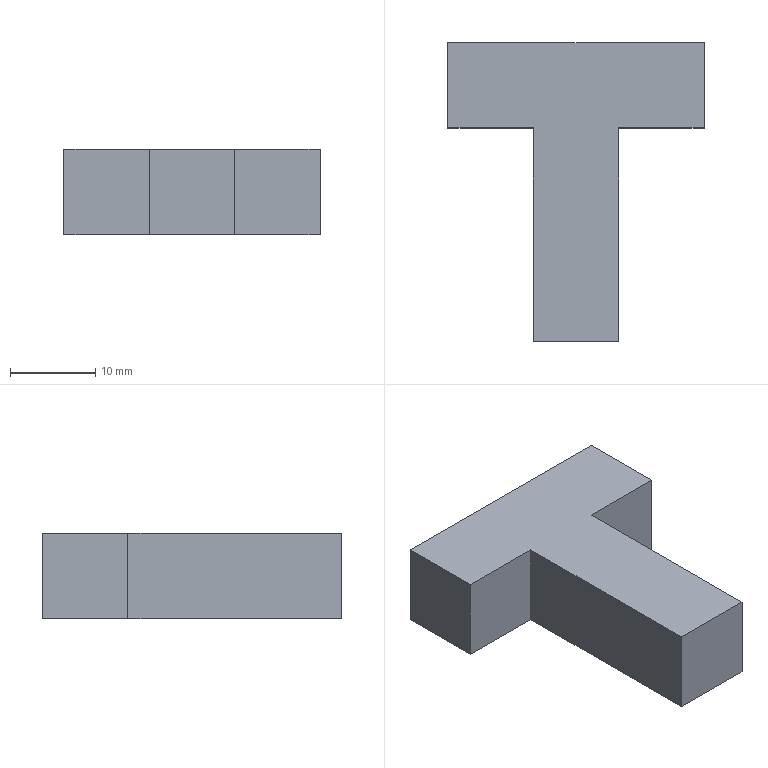Part | SolidWorks | features Extrusion 1, ICE 1 | 1 solid | 10 faces | box 30 x 35 x 10 mm | volume 5500 mm3 | plane 10
STEP:
#1=CARTESIAN_POINT('',(-15.,17.5,0.));
#2=VERTEX_POINT('',#1);
#3=CARTESIAN_POINT('',(-15.,7.5,0.));
#4=VERTEX_POINT('',#3);
#5=CARTESIAN_POINT('',(-15.,17.5,0.));
#6=DIRECTION('',(0.,-1.,0.));
#7=VECTOR('',#6,1000.);
#8=LINE('',#5,#7);
#9=EDGE_CURVE('',#2,#4,#8,.T.);
#10=ORIENTED_EDGE('',*,*,#9,.T.);
#11=CARTESIAN_POINT('',(-15.,7.5,10.));
#12=VERTEX_POINT('',#11);
#13=CARTESIAN_POINT('',(-15.,7.5,0.));
#14=DIRECTION('',(0.,0.,1.));
#15=VECTOR('',#14,1000.);
#16=LINE('',#13,#15);
#17=EDGE_CURVE('',#4,#12,#16,.T.);
#18=ORIENTED_EDGE('',*,*,#17,.T.);
#19=CARTESIAN_POINT('',(-15.,17.5,10.));
#20=VERTEX_POINT('',#19);
#21=CARTESIAN_POINT('',(-15.,17.5,10.));
#22=DIRECTION('',(0.,-1.,0.));
#23=VECTOR('',#22,1000.);
#24=LINE('',#21,#23);
#25=EDGE_CURVE('',#20,#12,#24,.T.);
#26=ORIENTED_EDGE('',*,*,#25,.F.);
#27=CARTESIAN_POINT('',(-15.,17.5,10.));
#28=DIRECTION('',(0.,0.,-1.));
#29=VECTOR('',#28,1000.);
#30=LINE('',#27,#29);
#31=EDGE_CURVE('',#20,#2,#30,.T.);
#32=ORIENTED_EDGE('',*,*,#31,.T.);
#33=EDGE_LOOP('',(#10,#18,#26,#32));
#34=FACE_OUTER_BOUND('',#33,.T.);
#35=CARTESIAN_POINT('',(-15.,17.5,10.));
#36=DIRECTION('',(1.,0.,0.));
#37=DIRECTION('',(0.,1.,0.));
#38=AXIS2_PLACEMENT_3D('',#35,#36,#37);
#39=PLANE('',#38);
#40=ADVANCED_FACE('',(#34),#39,.F.);
#41=CARTESIAN_POINT('',(-5.,-17.5,0.));
#42=VERTEX_POINT('',#41);
#43=CARTESIAN_POINT('',(5.,-17.5,0.));
#44=VERTEX_POINT('',#43);
#45=CARTESIAN_POINT('',(-15.,-17.5,0.));
#46=DIRECTION('',(1.,0.,0.));
#47=VECTOR('',#46,1000.);
#48=LINE('',#45,#47);
#49=EDGE_CURVE('',#42,#44,#48,.T.);
#50=ORIENTED_EDGE('',*,*,#49,.T.);
#51=CARTESIAN_POINT('',(5.,-17.5,10.));
#52=VERTEX_POINT('',#51);
#53=CARTESIAN_POINT('',(5.,-17.5,0.));
#54=DIRECTION('',(0.,0.,1.));
#55=VECTOR('',#54,1000.);
#56=LINE('',#53,#55);
#57=EDGE_CURVE('',#44,#52,#56,.T.);
#58=ORIENTED_EDGE('',*,*,#57,.T.);
#59=CARTESIAN_POINT('',(-5.,-17.5,10.));
#60=VERTEX_POINT('',#59);
#61=CARTESIAN_POINT('',(-15.,-17.5,10.));
#62=DIRECTION('',(1.,0.,0.));
#63=VECTOR('',#62,1000.);
#64=LINE('',#61,#63);
#65=EDGE_CURVE('',#60,#52,#64,.T.);
#66=ORIENTED_EDGE('',*,*,#65,.F.);
#67=CARTESIAN_POINT('',(-5.,-17.5,0.));
#68=DIRECTION('',(0.,0.,1.));
#69=VECTOR('',#68,1000.);
#70=LINE('',#67,#69);
#71=EDGE_CURVE('',#42,#60,#70,.T.);
#72=ORIENTED_EDGE('',*,*,#71,.F.);
#73=EDGE_LOOP('',(#50,#58,#66,#72));
#74=FACE_OUTER_BOUND('',#73,.T.);
#75=CARTESIAN_POINT('',(-15.,-17.5,10.));
#76=DIRECTION('',(0.,1.,0.));
#77=DIRECTION('',(0.,0.,1.));
#78=AXIS2_PLACEMENT_3D('',#75,#76,#77);
#79=PLANE('',#78);
#80=ADVANCED_FACE('',(#74),#79,.F.);
#81=CARTESIAN_POINT('',(15.,7.5,10.));
#82=VERTEX_POINT('',#81);
#83=CARTESIAN_POINT('',(15.,17.5,10.));
#84=VERTEX_POINT('',#83);
#85=CARTESIAN_POINT('',(15.,17.5,10.));
#86=DIRECTION('',(0.,1.,0.));
#87=VECTOR('',#86,1000.);
#88=LINE('',#85,#87);
#89=EDGE_CURVE('',#82,#84,#88,.T.);
#90=ORIENTED_EDGE('',*,*,#89,.F.);
#91=CARTESIAN_POINT('',(15.,7.5,0.));
#92=VERTEX_POINT('',#91);
#93=CARTESIAN_POINT('',(15.,7.5,0.));
#94=DIRECTION('',(0.,0.,1.));
#95=VECTOR('',#94,1000.);
#96=LINE('',#93,#95);
#97=EDGE_CURVE('',#92,#82,#96,.T.);
#98=ORIENTED_EDGE('',*,*,#97,.F.);
#99=CARTESIAN_POINT('',(15.,17.5,0.));
#100=VERTEX_POINT('',#99);
#101=CARTESIAN_POINT('',(15.,17.5,0.));
#102=DIRECTION('',(0.,1.,0.));
#103=VECTOR('',#102,1000.);
#104=LINE('',#101,#103);
#105=EDGE_CURVE('',#92,#100,#104,.T.);
#106=ORIENTED_EDGE('',*,*,#105,.T.);
#107=CARTESIAN_POINT('',(15.,17.5,10.));
#108=DIRECTION('',(0.,0.,-1.));
#109=VECTOR('',#108,1000.);
#110=LINE('',#107,#109);
#111=EDGE_CURVE('',#84,#100,#110,.T.);
#112=ORIENTED_EDGE('',*,*,#111,.F.);
#113=EDGE_LOOP('',(#90,#98,#106,#112));
#114=FACE_OUTER_BOUND('',#113,.T.);
#115=CARTESIAN_POINT('',(15.,17.5,10.));
#116=DIRECTION('',(-1.,0.,0.));
#117=DIRECTION('',(0.,-1.,0.));
#118=AXIS2_PLACEMENT_3D('',#115,#116,#117);
#119=PLANE('',#118);
#120=ADVANCED_FACE('',(#114),#119,.F.);
#121=CARTESIAN_POINT('',(-15.,17.5,0.));
#122=DIRECTION('',(-1.,0.,0.));
#123=VECTOR('',#122,1000.);
#124=LINE('',#121,#123);
#125=EDGE_CURVE('',#100,#2,#124,.T.);
#126=ORIENTED_EDGE('',*,*,#125,.T.);
#127=ORIENTED_EDGE('',*,*,#31,.F.);
#128=CARTESIAN_POINT('',(-15.,17.5,10.));
#129=DIRECTION('',(-1.,0.,0.));
#130=VECTOR('',#129,1000.);
#131=LINE('',#128,#130);
#132=EDGE_CURVE('',#84,#20,#131,.T.);
#133=ORIENTED_EDGE('',*,*,#132,.F.);
#134=ORIENTED_EDGE('',*,*,#111,.T.);
#135=EDGE_LOOP('',(#126,#127,#133,#134));
#136=FACE_OUTER_BOUND('',#135,.T.);
#137=CARTESIAN_POINT('',(-15.,17.5,10.));
#138=DIRECTION('',(0.,-1.,0.));
#139=DIRECTION('',(0.,0.,-1.));
#140=AXIS2_PLACEMENT_3D('',#137,#138,#139);
#141=PLANE('',#140);
#142=ADVANCED_FACE('',(#136),#141,.F.);
#143=CARTESIAN_POINT('',(5.,7.5,10.));
#144=VERTEX_POINT('',#143);
#145=CARTESIAN_POINT('',(5.,-17.5,10.));
#146=DIRECTION('',(0.,-1.,0.));
#147=VECTOR('',#146,1000.);
#148=LINE('',#145,#147);
#149=EDGE_CURVE('',#144,#52,#148,.T.);
#150=ORIENTED_EDGE('',*,*,#149,.F.);
#151=CARTESIAN_POINT('',(15.,7.5,10.));
#152=DIRECTION('',(-1.,0.,0.));
#153=VECTOR('',#152,1000.);
#154=LINE('',#151,#153);
#155=EDGE_CURVE('',#82,#144,#154,.T.);
#156=ORIENTED_EDGE('',*,*,#155,.F.);
#157=ORIENTED_EDGE('',*,*,#89,.T.);
#158=ORIENTED_EDGE('',*,*,#132,.T.);
#159=ORIENTED_EDGE('',*,*,#25,.T.);
#160=CARTESIAN_POINT('',(-5.,7.5,10.));
#161=VERTEX_POINT('',#160);
#162=CARTESIAN_POINT('',(-15.,7.5,10.));
#163=DIRECTION('',(-1.,0.,0.));
#164=VECTOR('',#163,1000.);
#165=LINE('',#162,#164);
#166=EDGE_CURVE('',#161,#12,#165,.T.);
#167=ORIENTED_EDGE('',*,*,#166,.F.);
#168=CARTESIAN_POINT('',(-5.,-17.5,10.));
#169=DIRECTION('',(0.,1.,0.));
#170=VECTOR('',#169,1000.);
#171=LINE('',#168,#170);
#172=EDGE_CURVE('',#60,#161,#171,.T.);
#173=ORIENTED_EDGE('',*,*,#172,.F.);
#174=ORIENTED_EDGE('',*,*,#65,.T.);
#175=EDGE_LOOP('',(#150,#156,#157,#158,#159,#167,#173,#174));
#176=FACE_OUTER_BOUND('',#175,.T.);
#177=CARTESIAN_POINT('',(0.,0.,10.));
#178=DIRECTION('',(0.,0.,1.));
#179=DIRECTION('',(1.,0.,0.));
#180=AXIS2_PLACEMENT_3D('',#177,#178,#179);
#181=PLANE('',#180);
#182=ADVANCED_FACE('',(#176),#181,.T.);
#183=CARTESIAN_POINT('',(5.,7.5,0.));
#184=VERTEX_POINT('',#183);
#185=CARTESIAN_POINT('',(15.,7.5,0.));
#186=DIRECTION('',(-1.,0.,0.));
#187=VECTOR('',#186,1000.);
#188=LINE('',#185,#187);
#189=EDGE_CURVE('',#92,#184,#188,.T.);
#190=ORIENTED_EDGE('',*,*,#189,.T.);
#191=CARTESIAN_POINT('',(5.,-17.5,0.));
#192=DIRECTION('',(0.,-1.,0.));
#193=VECTOR('',#192,1000.);
#194=LINE('',#191,#193);
#195=EDGE_CURVE('',#184,#44,#194,.T.);
#196=ORIENTED_EDGE('',*,*,#195,.T.);
#197=ORIENTED_EDGE('',*,*,#49,.F.);
#198=CARTESIAN_POINT('',(-5.,7.5,0.));
#199=VERTEX_POINT('',#198);
#200=CARTESIAN_POINT('',(-5.,-17.5,0.));
#201=DIRECTION('',(0.,1.,0.));
#202=VECTOR('',#201,1000.);
#203=LINE('',#200,#202);
#204=EDGE_CURVE('',#42,#199,#203,.T.);
#205=ORIENTED_EDGE('',*,*,#204,.T.);
#206=CARTESIAN_POINT('',(-15.,7.5,0.));
#207=DIRECTION('',(-1.,0.,0.));
#208=VECTOR('',#207,1000.);
#209=LINE('',#206,#208);
#210=EDGE_CURVE('',#199,#4,#209,.T.);
#211=ORIENTED_EDGE('',*,*,#210,.T.);
#212=ORIENTED_EDGE('',*,*,#9,.F.);
#213=ORIENTED_EDGE('',*,*,#125,.F.);
#214=ORIENTED_EDGE('',*,*,#105,.F.);
#215=EDGE_LOOP('',(#190,#196,#197,#205,#211,#212,#213,#214));
#216=FACE_OUTER_BOUND('',#215,.T.);
#217=CARTESIAN_POINT('',(0.,0.,0.));
#218=DIRECTION('',(0.,0.,1.));
#219=DIRECTION('',(1.,0.,0.));
#220=AXIS2_PLACEMENT_3D('',#217,#218,#219);
#221=PLANE('',#220);
#222=ADVANCED_FACE('',(#216),#221,.F.);
#223=ORIENTED_EDGE('',*,*,#166,.T.);
#224=ORIENTED_EDGE('',*,*,#17,.F.);
#225=ORIENTED_EDGE('',*,*,#210,.F.);
#226=CARTESIAN_POINT('',(-5.,7.5,0.));
#227=DIRECTION('',(0.,0.,1.));
#228=VECTOR('',#227,1000.);
#229=LINE('',#226,#228);
#230=EDGE_CURVE('',#199,#161,#229,.T.);
#231=ORIENTED_EDGE('',*,*,#230,.T.);
#232=EDGE_LOOP('',(#223,#224,#225,#231));
#233=FACE_OUTER_BOUND('',#232,.T.);
#234=CARTESIAN_POINT('',(-15.,7.5,0.));
#235=DIRECTION('',(0.,1.,0.));
#236=DIRECTION('',(0.,0.,1.));
#237=AXIS2_PLACEMENT_3D('',#234,#235,#236);
#238=PLANE('',#237);
#239=ADVANCED_FACE('',(#233),#238,.F.);
#240=ORIENTED_EDGE('',*,*,#172,.T.);
#241=ORIENTED_EDGE('',*,*,#230,.F.);
#242=ORIENTED_EDGE('',*,*,#204,.F.);
#243=ORIENTED_EDGE('',*,*,#71,.T.);
#244=EDGE_LOOP('',(#240,#241,#242,#243));
#245=FACE_OUTER_BOUND('',#244,.T.);
#246=CARTESIAN_POINT('',(-5.,-17.5,0.));
#247=DIRECTION('',(1.,0.,0.));
#248=DIRECTION('',(0.,0.,-1.));
#249=AXIS2_PLACEMENT_3D('',#246,#247,#248);
#250=PLANE('',#249);
#251=ADVANCED_FACE('',(#245),#250,.F.);
#252=ORIENTED_EDGE('',*,*,#149,.T.);
#253=ORIENTED_EDGE('',*,*,#57,.F.);
#254=ORIENTED_EDGE('',*,*,#195,.F.);
#255=CARTESIAN_POINT('',(5.,7.5,0.));
#256=DIRECTION('',(0.,0.,1.));
#257=VECTOR('',#256,1000.);
#258=LINE('',#255,#257);
#259=EDGE_CURVE('',#184,#144,#258,.T.);
#260=ORIENTED_EDGE('',*,*,#259,.T.);
#261=EDGE_LOOP('',(#252,#253,#254,#260));
#262=FACE_OUTER_BOUND('',#261,.T.);
#263=CARTESIAN_POINT('',(5.,-17.5,0.));
#264=DIRECTION('',(-1.,0.,0.));
#265=DIRECTION('',(0.,0.,1.));
#266=AXIS2_PLACEMENT_3D('',#263,#264,#265);
#267=PLANE('',#266);
#268=ADVANCED_FACE('',(#262),#267,.F.);
#269=ORIENTED_EDGE('',*,*,#155,.T.);
#270=ORIENTED_EDGE('',*,*,#259,.F.);
#271=ORIENTED_EDGE('',*,*,#189,.F.);
#272=ORIENTED_EDGE('',*,*,#97,.T.);
#273=EDGE_LOOP('',(#269,#270,#271,#272));
#274=FACE_OUTER_BOUND('',#273,.T.);
#275=CARTESIAN_POINT('',(15.,7.5,0.));
#276=DIRECTION('',(0.,1.,0.));
#277=DIRECTION('',(0.,0.,1.));
#278=AXIS2_PLACEMENT_3D('',#275,#276,#277);
#279=PLANE('',#278);
#280=ADVANCED_FACE('',(#274),#279,.F.);
#281=CLOSED_SHELL('',(#40,#80,#120,#142,#182,#222,#239,#251,#268,#280));
#282=MANIFOLD_SOLID_BREP('',#281);
#283=CARTESIAN_POINT('',(0.,0.,0.));
#284=DIRECTION('',(0.,0.,1.));
#285=DIRECTION('',(1.,0.,0.));
#286=AXIS2_PLACEMENT_3D('',#283,#284,#285);
#287=(LENGTH_UNIT()NAMED_UNIT(*)SI_UNIT(.MILLI.,.METRE.));
#288=UNCERTAINTY_MEASURE_WITH_UNIT(LENGTH_MEASURE(0.00001),#287,'','');
#289=(NAMED_UNIT(*)PLANE_ANGLE_UNIT()SI_UNIT($,.RADIAN.));
#290=(NAMED_UNIT(*)SI_UNIT($,.STERADIAN.)SOLID_ANGLE_UNIT());
#291=(GEOMETRIC_REPRESENTATION_CONTEXT(3)GLOBAL_UNCERTAINTY_ASSIGNED_CONTEXT((#288))GLOBAL_UNIT_ASSIGNED_CONTEXT((#287,#289,#290))REPRESENTATION_CONTEXT('',''));
#292=ADVANCED_BREP_SHAPE_REPRESENTATION('',(#282,#286),#291);